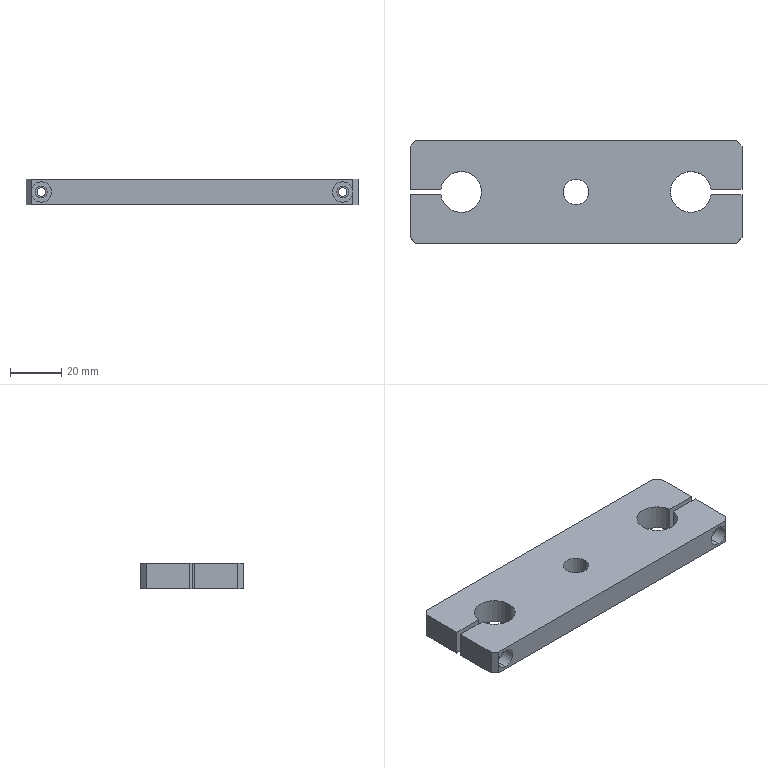Part | STEP file | Cylinder fixing plate 1 | 1 solid | 35 faces | box 130 x 40 x 10 mm | volume 45360 mm3 | plane 18 | cylinder 17 | commonest cylinder face diameters 3.3 x4 4.5 x4 8 x4 16 x3 10 x2